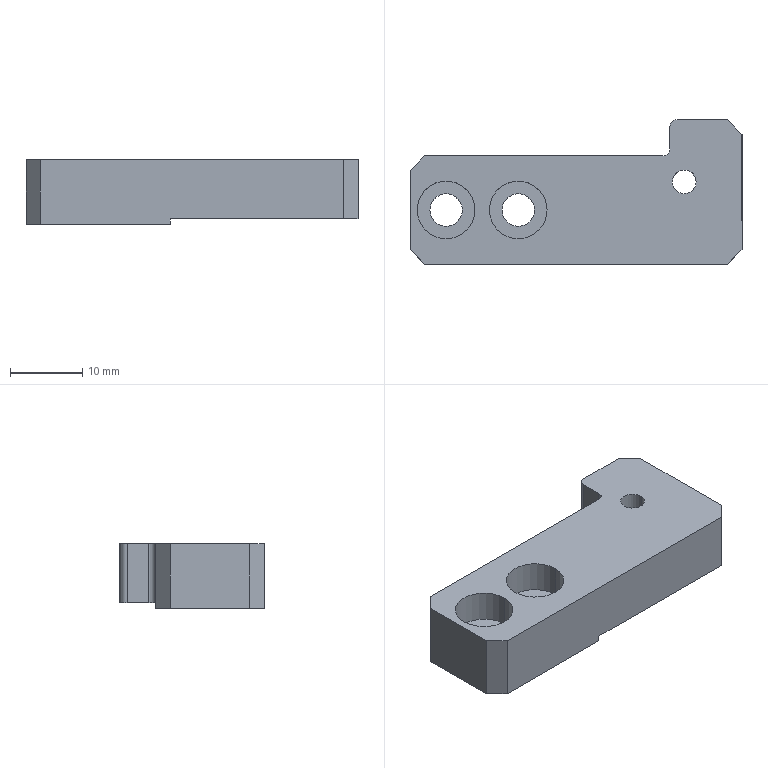Part | STEP file | 11-FG-B03811 | 1 solid | 28 faces | box 46 x 20 x 9 mm | volume 5580 mm3 | plane 16 | cylinder 12 | commonest cylinder face diameters 4.5 x4 8 x4 2 x2 3.3 x2
STEP:
#1=CARTESIAN_POINT('',(1.,7.5,4.6));
#2=VERTEX_POINT('',#1);
#3=CARTESIAN_POINT('',(9.,7.5,4.6));
#4=VERTEX_POINT('',#3);
#5=CARTESIAN_POINT('',(5.,7.5,4.6));
#6=DIRECTION('',(0.,0.,1.));
#7=DIRECTION('',(1.,0.,0.));
#8=AXIS2_PLACEMENT_3D('',#5,#6,#7);
#9=CIRCLE('',#8,4.);
#10=EDGE_CURVE('',#2,#4,#9,.T.);
#11=ORIENTED_EDGE('',*,*,#10,.F.);
#12=CARTESIAN_POINT('',(1.,7.5,9.));
#13=VERTEX_POINT('',#12);
#14=CARTESIAN_POINT('',(1.,7.5,9.));
#15=DIRECTION('',(0.,0.,1.));
#16=VECTOR('',#15,1000.);
#17=LINE('',#14,#16);
#18=EDGE_CURVE('',#2,#13,#17,.T.);
#19=ORIENTED_EDGE('',*,*,#18,.T.);
#20=CARTESIAN_POINT('',(9.,7.5,9.));
#21=VERTEX_POINT('',#20);
#22=CARTESIAN_POINT('',(5.,7.5,9.));
#23=DIRECTION('',(0.,0.,1.));
#24=DIRECTION('',(1.,0.,0.));
#25=AXIS2_PLACEMENT_3D('',#22,#23,#24);
#26=CIRCLE('',#25,4.);
#27=EDGE_CURVE('',#13,#21,#26,.T.);
#28=ORIENTED_EDGE('',*,*,#27,.T.);
#29=CARTESIAN_POINT('',(9.,7.5,9.));
#30=DIRECTION('',(0.,0.,1.));
#31=VECTOR('',#30,1000.);
#32=LINE('',#29,#31);
#33=EDGE_CURVE('',#4,#21,#32,.T.);
#34=ORIENTED_EDGE('',*,*,#33,.F.);
#35=EDGE_LOOP('',(#11,#19,#28,#34));
#36=FACE_OUTER_BOUND('',#35,.T.);
#37=CARTESIAN_POINT('',(5.,7.5,9.));
#38=DIRECTION('',(0.,0.,1.));
#39=DIRECTION('',(1.,0.,0.));
#40=AXIS2_PLACEMENT_3D('',#37,#38,#39);
#41=CYLINDRICAL_SURFACE('',#40,4.);
#42=ADVANCED_FACE('',(#36),#41,.F.);
#43=CARTESIAN_POINT('',(7.25,7.5,0.));
#44=VERTEX_POINT('',#43);
#45=CARTESIAN_POINT('',(2.75,7.5,0.));
#46=VERTEX_POINT('',#45);
#47=CARTESIAN_POINT('',(5.,7.5,0.));
#48=DIRECTION('',(0.,0.,-1.));
#49=DIRECTION('',(-1.,0.,0.));
#50=AXIS2_PLACEMENT_3D('',#47,#48,#49);
#51=CIRCLE('',#50,2.25);
#52=EDGE_CURVE('',#44,#46,#51,.T.);
#53=ORIENTED_EDGE('',*,*,#52,.T.);
#54=CARTESIAN_POINT('',(2.75,7.5,4.6));
#55=VERTEX_POINT('',#54);
#56=CARTESIAN_POINT('',(2.75,7.5,9.));
#57=DIRECTION('',(0.,0.,1.));
#58=VECTOR('',#57,1000.);
#59=LINE('',#56,#58);
#60=EDGE_CURVE('',#46,#55,#59,.T.);
#61=ORIENTED_EDGE('',*,*,#60,.T.);
#62=CARTESIAN_POINT('',(7.25,7.5,4.6));
#63=VERTEX_POINT('',#62);
#64=CARTESIAN_POINT('',(5.,7.5,4.6));
#65=DIRECTION('',(0.,0.,1.));
#66=DIRECTION('',(1.,0.,0.));
#67=AXIS2_PLACEMENT_3D('',#64,#65,#66);
#68=CIRCLE('',#67,2.25);
#69=EDGE_CURVE('',#55,#63,#68,.T.);
#70=ORIENTED_EDGE('',*,*,#69,.T.);
#71=CARTESIAN_POINT('',(7.25,7.5,9.));
#72=DIRECTION('',(0.,0.,1.));
#73=VECTOR('',#72,1000.);
#74=LINE('',#71,#73);
#75=EDGE_CURVE('',#44,#63,#74,.T.);
#76=ORIENTED_EDGE('',*,*,#75,.F.);
#77=EDGE_LOOP('',(#53,#61,#70,#76));
#78=FACE_OUTER_BOUND('',#77,.T.);
#79=CARTESIAN_POINT('',(5.,7.5,9.));
#80=DIRECTION('',(0.,0.,1.));
#81=DIRECTION('',(1.,0.,0.));
#82=AXIS2_PLACEMENT_3D('',#79,#80,#81);
#83=CYLINDRICAL_SURFACE('',#82,2.25);
#84=ADVANCED_FACE('',(#78),#83,.F.);
#85=CARTESIAN_POINT('',(11.,7.5,4.6));
#86=VERTEX_POINT('',#85);
#87=CARTESIAN_POINT('',(19.,7.5,4.6));
#88=VERTEX_POINT('',#87);
#89=CARTESIAN_POINT('',(15.,7.5,4.6));
#90=DIRECTION('',(0.,0.,1.));
#91=DIRECTION('',(1.,0.,0.));
#92=AXIS2_PLACEMENT_3D('',#89,#90,#91);
#93=CIRCLE('',#92,4.);
#94=EDGE_CURVE('',#86,#88,#93,.T.);
#95=ORIENTED_EDGE('',*,*,#94,.F.);
#96=CARTESIAN_POINT('',(11.,7.5,9.));
#97=VERTEX_POINT('',#96);
#98=CARTESIAN_POINT('',(11.,7.5,9.));
#99=DIRECTION('',(0.,0.,1.));
#100=VECTOR('',#99,1000.);
#101=LINE('',#98,#100);
#102=EDGE_CURVE('',#86,#97,#101,.T.);
#103=ORIENTED_EDGE('',*,*,#102,.T.);
#104=CARTESIAN_POINT('',(19.,7.5,9.));
#105=VERTEX_POINT('',#104);
#106=CARTESIAN_POINT('',(15.,7.5,9.));
#107=DIRECTION('',(0.,0.,1.));
#108=DIRECTION('',(1.,0.,0.));
#109=AXIS2_PLACEMENT_3D('',#106,#107,#108);
#110=CIRCLE('',#109,4.);
#111=EDGE_CURVE('',#97,#105,#110,.T.);
#112=ORIENTED_EDGE('',*,*,#111,.T.);
#113=CARTESIAN_POINT('',(19.,7.5,9.));
#114=DIRECTION('',(0.,0.,1.));
#115=VECTOR('',#114,1000.);
#116=LINE('',#113,#115);
#117=EDGE_CURVE('',#88,#105,#116,.T.);
#118=ORIENTED_EDGE('',*,*,#117,.F.);
#119=EDGE_LOOP('',(#95,#103,#112,#118));
#120=FACE_OUTER_BOUND('',#119,.T.);
#121=CARTESIAN_POINT('',(15.,7.5,9.));
#122=DIRECTION('',(0.,0.,1.));
#123=DIRECTION('',(1.,0.,0.));
#124=AXIS2_PLACEMENT_3D('',#121,#122,#123);
#125=CYLINDRICAL_SURFACE('',#124,4.);
#126=ADVANCED_FACE('',(#120),#125,.F.);
#127=CARTESIAN_POINT('',(17.25,7.5,0.));
#128=VERTEX_POINT('',#127);
#129=CARTESIAN_POINT('',(12.75,7.5,0.));
#130=VERTEX_POINT('',#129);
#131=CARTESIAN_POINT('',(15.,7.5,0.));
#132=DIRECTION('',(0.,0.,-1.));
#133=DIRECTION('',(-1.,0.,0.));
#134=AXIS2_PLACEMENT_3D('',#131,#132,#133);
#135=CIRCLE('',#134,2.25);
#136=EDGE_CURVE('',#128,#130,#135,.T.);
#137=ORIENTED_EDGE('',*,*,#136,.T.);
#138=CARTESIAN_POINT('',(12.75,7.5,4.6));
#139=VERTEX_POINT('',#138);
#140=CARTESIAN_POINT('',(12.75,7.5,9.));
#141=DIRECTION('',(0.,0.,1.));
#142=VECTOR('',#141,1000.);
#143=LINE('',#140,#142);
#144=EDGE_CURVE('',#130,#139,#143,.T.);
#145=ORIENTED_EDGE('',*,*,#144,.T.);
#146=CARTESIAN_POINT('',(17.25,7.5,4.6));
#147=VERTEX_POINT('',#146);
#148=CARTESIAN_POINT('',(15.,7.5,4.6));
#149=DIRECTION('',(0.,0.,1.));
#150=DIRECTION('',(1.,0.,0.));
#151=AXIS2_PLACEMENT_3D('',#148,#149,#150);
#152=CIRCLE('',#151,2.25);
#153=EDGE_CURVE('',#139,#147,#152,.T.);
#154=ORIENTED_EDGE('',*,*,#153,.T.);
#155=CARTESIAN_POINT('',(17.25,7.5,9.));
#156=DIRECTION('',(0.,0.,1.));
#157=VECTOR('',#156,1000.);
#158=LINE('',#155,#157);
#159=EDGE_CURVE('',#128,#147,#158,.T.);
#160=ORIENTED_EDGE('',*,*,#159,.F.);
#161=EDGE_LOOP('',(#137,#145,#154,#160));
#162=FACE_OUTER_BOUND('',#161,.T.);
#163=CARTESIAN_POINT('',(15.,7.5,9.));
#164=DIRECTION('',(0.,0.,1.));
#165=DIRECTION('',(1.,0.,0.));
#166=AXIS2_PLACEMENT_3D('',#163,#164,#165);
#167=CYLINDRICAL_SURFACE('',#166,2.25);
#168=ADVANCED_FACE('',(#162),#167,.F.);
#169=CARTESIAN_POINT('',(39.65,11.4,9.));
#170=VERTEX_POINT('',#169);
#171=CARTESIAN_POINT('',(36.35,11.4,9.));
#172=VERTEX_POINT('',#171);
#173=CARTESIAN_POINT('',(38.,11.4,9.));
#174=DIRECTION('',(0.,0.,-1.));
#175=DIRECTION('',(-1.,0.,0.));
#176=AXIS2_PLACEMENT_3D('',#173,#174,#175);
#177=CIRCLE('',#176,1.65);
#178=EDGE_CURVE('',#170,#172,#177,.T.);
#179=ORIENTED_EDGE('',*,*,#178,.F.);
#180=CARTESIAN_POINT('',(39.65,11.4,0.8));
#181=VERTEX_POINT('',#180);
#182=CARTESIAN_POINT('',(39.65,11.4,0.));
#183=DIRECTION('',(0.,0.,-1.));
#184=VECTOR('',#183,1000.);
#185=LINE('',#182,#184);
#186=EDGE_CURVE('',#170,#181,#185,.T.);
#187=ORIENTED_EDGE('',*,*,#186,.T.);
#188=CARTESIAN_POINT('',(36.35,11.4,0.8));
#189=VERTEX_POINT('',#188);
#190=CARTESIAN_POINT('',(38.,11.4,0.8));
#191=DIRECTION('',(0.,0.,-1.));
#192=DIRECTION('',(1.,0.,0.));
#193=AXIS2_PLACEMENT_3D('',#190,#191,#192);
#194=CIRCLE('',#193,1.65);
#195=EDGE_CURVE('',#181,#189,#194,.T.);
#196=ORIENTED_EDGE('',*,*,#195,.T.);
#197=CARTESIAN_POINT('',(36.35,11.4,0.));
#198=DIRECTION('',(0.,0.,-1.));
#199=VECTOR('',#198,1000.);
#200=LINE('',#197,#199);
#201=EDGE_CURVE('',#172,#189,#200,.T.);
#202=ORIENTED_EDGE('',*,*,#201,.F.);
#203=EDGE_LOOP('',(#179,#187,#196,#202));
#204=FACE_OUTER_BOUND('',#203,.T.);
#205=CARTESIAN_POINT('',(38.,11.4,0.));
#206=DIRECTION('',(0.,0.,-1.));
#207=DIRECTION('',(-1.,0.,0.));
#208=AXIS2_PLACEMENT_3D('',#205,#206,#207);
#209=CYLINDRICAL_SURFACE('',#208,1.65);
#210=ADVANCED_FACE('',(#204),#209,.F.);
#211=CARTESIAN_POINT('',(0.,13.,9.));
#212=VERTEX_POINT('',#211);
#213=CARTESIAN_POINT('',(0.,2.,9.));
#214=VERTEX_POINT('',#213);
#215=CARTESIAN_POINT('',(0.,0.,9.));
#216=DIRECTION('',(0.,-1.,0.));
#217=VECTOR('',#216,1000.);
#218=LINE('',#215,#217);
#219=EDGE_CURVE('',#212,#214,#218,.T.);
#220=ORIENTED_EDGE('',*,*,#219,.F.);
#221=CARTESIAN_POINT('',(0.,13.,0.));
#222=VERTEX_POINT('',#221);
#223=CARTESIAN_POINT('',(0.,13.,9.));
#224=DIRECTION('',(0.,0.,-1.));
#225=VECTOR('',#224,1000.);
#226=LINE('',#223,#225);
#227=EDGE_CURVE('',#212,#222,#226,.T.);
#228=ORIENTED_EDGE('',*,*,#227,.T.);
#229=CARTESIAN_POINT('',(0.,2.,0.));
#230=VERTEX_POINT('',#229);
#231=CARTESIAN_POINT('',(0.,0.,0.));
#232=DIRECTION('',(0.,-1.,0.));
#233=VECTOR('',#232,1000.);
#234=LINE('',#231,#233);
#235=EDGE_CURVE('',#222,#230,#234,.T.);
#236=ORIENTED_EDGE('',*,*,#235,.T.);
#237=CARTESIAN_POINT('',(0.,2.,9.));
#238=DIRECTION('',(0.,0.,1.));
#239=VECTOR('',#238,1000.);
#240=LINE('',#237,#239);
#241=EDGE_CURVE('',#230,#214,#240,.T.);
#242=ORIENTED_EDGE('',*,*,#241,.T.);
#243=EDGE_LOOP('',(#220,#228,#236,#242));
#244=FACE_OUTER_BOUND('',#243,.T.);
#245=CARTESIAN_POINT('',(0.,0.,9.));
#246=DIRECTION('',(1.,0.,0.));
#247=DIRECTION('',(0.,1.,0.));
#248=AXIS2_PLACEMENT_3D('',#245,#246,#247);
#249=PLANE('',#248);
#250=ADVANCED_FACE('',(#244),#249,.F.);
#251=CARTESIAN_POINT('',(2.,0.,0.));
#252=VERTEX_POINT('',#251);
#253=CARTESIAN_POINT('',(20.,0.,0.));
#254=VERTEX_POINT('',#253);
#255=CARTESIAN_POINT('',(0.,0.,0.));
#256=DIRECTION('',(1.,0.,0.));
#257=VECTOR('',#256,1000.);
#258=LINE('',#255,#257);
#259=EDGE_CURVE('',#252,#254,#258,.T.);
#260=ORIENTED_EDGE('',*,*,#259,.T.);
#261=CARTESIAN_POINT('',(20.,0.,0.8));
#262=VERTEX_POINT('',#261);
#263=CARTESIAN_POINT('',(20.,0.,0.));
#264=DIRECTION('',(0.,0.,-1.));
#265=VECTOR('',#264,1000.);
#266=LINE('',#263,#265);
#267=EDGE_CURVE('',#262,#254,#266,.T.);
#268=ORIENTED_EDGE('',*,*,#267,.F.);
#269=CARTESIAN_POINT('',(44.,0.,0.8));
#270=VERTEX_POINT('',#269);
#271=CARTESIAN_POINT('',(46.,0.,0.8));
#272=DIRECTION('',(-1.,0.,0.));
#273=VECTOR('',#272,1000.);
#274=LINE('',#271,#273);
#275=EDGE_CURVE('',#270,#262,#274,.T.);
#276=ORIENTED_EDGE('',*,*,#275,.F.);
#277=CARTESIAN_POINT('',(44.,0.,9.));
#278=VERTEX_POINT('',#277);
#279=CARTESIAN_POINT('',(44.,0.,9.));
#280=DIRECTION('',(0.,0.,1.));
#281=VECTOR('',#280,1000.);
#282=LINE('',#279,#281);
#283=EDGE_CURVE('',#270,#278,#282,.T.);
#284=ORIENTED_EDGE('',*,*,#283,.T.);
#285=CARTESIAN_POINT('',(2.,0.,9.));
#286=VERTEX_POINT('',#285);
#287=CARTESIAN_POINT('',(0.,0.,9.));
#288=DIRECTION('',(1.,0.,0.));
#289=VECTOR('',#288,1000.);
#290=LINE('',#287,#289);
#291=EDGE_CURVE('',#286,#278,#290,.T.);
#292=ORIENTED_EDGE('',*,*,#291,.F.);
#293=CARTESIAN_POINT('',(2.,0.,9.));
#294=DIRECTION('',(0.,0.,-1.));
#295=VECTOR('',#294,1000.);
#296=LINE('',#293,#295);
#297=EDGE_CURVE('',#286,#252,#296,.T.);
#298=ORIENTED_EDGE('',*,*,#297,.T.);
#299=EDGE_LOOP('',(#260,#268,#276,#284,#292,#298));
#300=FACE_OUTER_BOUND('',#299,.T.);
#301=CARTESIAN_POINT('',(0.,0.,9.));
#302=DIRECTION('',(0.,1.,0.));
#303=DIRECTION('',(0.,0.,1.));
#304=AXIS2_PLACEMENT_3D('',#301,#302,#303);
#305=PLANE('',#304);
#306=ADVANCED_FACE('',(#300),#305,.F.);
#307=CARTESIAN_POINT('',(46.,2.,9.));
#308=VERTEX_POINT('',#307);
#309=CARTESIAN_POINT('',(46.,2.,0.8));
#310=VERTEX_POINT('',#309);
#311=CARTESIAN_POINT('',(46.,2.,9.));
#312=DIRECTION('',(0.,0.,-1.));
#313=VECTOR('',#312,1000.);
#314=LINE('',#311,#313);
#315=EDGE_CURVE('',#308,#310,#314,.T.);
#316=ORIENTED_EDGE('',*,*,#315,.T.);
#317=CARTESIAN_POINT('',(46.,18.,0.8));
#318=VERTEX_POINT('',#317);
#319=CARTESIAN_POINT('',(46.,29.,0.8));
#320=DIRECTION('',(0.,-1.,0.));
#321=VECTOR('',#320,1000.);
#322=LINE('',#319,#321);
#323=EDGE_CURVE('',#318,#310,#322,.T.);
#324=ORIENTED_EDGE('',*,*,#323,.F.);
#325=CARTESIAN_POINT('',(46.,18.,9.));
#326=VERTEX_POINT('',#325);
#327=CARTESIAN_POINT('',(46.,18.,9.));
#328=DIRECTION('',(0.,0.,1.));
#329=VECTOR('',#328,1000.);
#330=LINE('',#327,#329);
#331=EDGE_CURVE('',#318,#326,#330,.T.);
#332=ORIENTED_EDGE('',*,*,#331,.T.);
#333=CARTESIAN_POINT('',(46.,0.,9.));
#334=DIRECTION('',(0.,1.,0.));
#335=VECTOR('',#334,1000.);
#336=LINE('',#333,#335);
#337=EDGE_CURVE('',#308,#326,#336,.T.);
#338=ORIENTED_EDGE('',*,*,#337,.F.);
#339=EDGE_LOOP('',(#316,#324,#332,#338));
#340=FACE_OUTER_BOUND('',#339,.T.);
#341=CARTESIAN_POINT('',(46.,0.,9.));
#342=DIRECTION('',(-1.,0.,0.));
#343=DIRECTION('',(0.,-1.,0.));
#344=AXIS2_PLACEMENT_3D('',#341,#342,#343);
#345=PLANE('',#344);
#346=ADVANCED_FACE('',(#340),#345,.F.);
#347=CARTESIAN_POINT('',(44.,20.,0.8));
#348=VERTEX_POINT('',#347);
#349=CARTESIAN_POINT('',(37.,20.,0.8));
#350=VERTEX_POINT('',#349);
#351=CARTESIAN_POINT('',(0.,20.,0.8));
#352=DIRECTION('',(-1.,0.,0.));
#353=VECTOR('',#352,1000.);
#354=LINE('',#351,#353);
#355=EDGE_CURVE('',#348,#350,#354,.T.);
#356=ORIENTED_EDGE('',*,*,#355,.T.);
#357=CARTESIAN_POINT('',(37.,20.,9.));
#358=VERTEX_POINT('',#357);
#359=CARTESIAN_POINT('',(37.,20.,9.));
#360=DIRECTION('',(0.,0.,1.));
#361=VECTOR('',#360,1000.);
#362=LINE('',#359,#361);
#363=EDGE_CURVE('',#350,#358,#362,.T.);
#364=ORIENTED_EDGE('',*,*,#363,.T.);
#365=CARTESIAN_POINT('',(44.,20.,9.));
#366=VERTEX_POINT('',#365);
#367=CARTESIAN_POINT('',(0.,20.,9.));
#368=DIRECTION('',(-1.,0.,0.));
#369=VECTOR('',#368,1000.);
#370=LINE('',#367,#369);
#371=EDGE_CURVE('',#366,#358,#370,.T.);
#372=ORIENTED_EDGE('',*,*,#371,.F.);
#373=CARTESIAN_POINT('',(44.,20.,9.));
#374=DIRECTION('',(0.,0.,-1.));
#375=VECTOR('',#374,1000.);
#376=LINE('',#373,#375);
#377=EDGE_CURVE('',#366,#348,#376,.T.);
#378=ORIENTED_EDGE('',*,*,#377,.T.);
#379=EDGE_LOOP('',(#356,#364,#372,#378));
#380=FACE_OUTER_BOUND('',#379,.T.);
#381=CARTESIAN_POINT('',(0.,20.,9.));
#382=DIRECTION('',(0.,-1.,0.));
#383=DIRECTION('',(0.,0.,-1.));
#384=AXIS2_PLACEMENT_3D('',#381,#382,#383);
#385=PLANE('',#384);
#386=ADVANCED_FACE('',(#380),#385,.F.);
#387=CARTESIAN_POINT('',(5.,7.5,9.));
#388=DIRECTION('',(0.,0.,1.));
#389=DIRECTION('',(1.,0.,0.));
#390=AXIS2_PLACEMENT_3D('',#387,#388,#389);
#391=CIRCLE('',#390,4.);
#392=EDGE_CURVE('',#21,#13,#391,.T.);
#393=ORIENTED_EDGE('',*,*,#392,.F.);
#394=ORIENTED_EDGE('',*,*,#27,.F.);
#395=EDGE_LOOP('',(#393,#394));
#396=FACE_BOUND('',#395,.T.);
#397=CARTESIAN_POINT('',(15.,7.5,9.));
#398=DIRECTION('',(0.,0.,1.));
#399=DIRECTION('',(1.,0.,0.));
#400=AXIS2_PLACEMENT_3D('',#397,#398,#399);
#401=CIRCLE('',#400,4.);
#402=EDGE_CURVE('',#105,#97,#401,.T.);
#403=ORIENTED_EDGE('',*,*,#402,.F.);
#404=ORIENTED_EDGE('',*,*,#111,.F.);
#405=EDGE_LOOP('',(#403,#404));
#406=FACE_BOUND('',#405,.T.);
#407=CARTESIAN_POINT('',(38.,11.4,9.));
#408=DIRECTION('',(0.,0.,-1.));
#409=DIRECTION('',(-1.,0.,0.));
#410=AXIS2_PLACEMENT_3D('',#407,#408,#409);
#411=CIRCLE('',#410,1.65);
#412=EDGE_CURVE('',#172,#170,#411,.T.);
#413=ORIENTED_EDGE('',*,*,#412,.T.);
#414=ORIENTED_EDGE('',*,*,#178,.T.);
#415=EDGE_LOOP('',(#413,#414));
#416=FACE_BOUND('',#415,.T.);
#417=ORIENTED_EDGE('',*,*,#371,.T.);
#418=CARTESIAN_POINT('',(36.,19.,9.));
#419=VERTEX_POINT('',#418);
#420=CARTESIAN_POINT('',(37.,19.,9.));
#421=DIRECTION('',(0.,0.,1.));
#422=DIRECTION('',(-1.,0.,0.));
#423=AXIS2_PLACEMENT_3D('',#420,#421,#422);
#424=CIRCLE('',#423,1.);
#425=EDGE_CURVE('',#358,#419,#424,.T.);
#426=ORIENTED_EDGE('',*,*,#425,.T.);
#427=CARTESIAN_POINT('',(36.,16.,9.));
#428=VERTEX_POINT('',#427);
#429=CARTESIAN_POINT('',(36.,15.,9.));
#430=DIRECTION('',(0.,1.,0.));
#431=VECTOR('',#430,1000.);
#432=LINE('',#429,#431);
#433=EDGE_CURVE('',#428,#419,#432,.T.);
#434=ORIENTED_EDGE('',*,*,#433,.F.);
#435=CARTESIAN_POINT('',(35.,15.,9.));
#436=VERTEX_POINT('',#435);
#437=CARTESIAN_POINT('',(35.,16.,9.));
#438=DIRECTION('',(0.,0.,-1.));
#439=DIRECTION('',(-1.,0.,0.));
#440=AXIS2_PLACEMENT_3D('',#437,#438,#439);
#441=CIRCLE('',#440,1.);
#442=EDGE_CURVE('',#428,#436,#441,.T.);
#443=ORIENTED_EDGE('',*,*,#442,.T.);
#444=CARTESIAN_POINT('',(2.,15.,9.));
#445=VERTEX_POINT('',#444);
#446=CARTESIAN_POINT('',(0.,15.,9.));
#447=DIRECTION('',(1.,0.,0.));
#448=VECTOR('',#447,1000.);
#449=LINE('',#446,#448);
#450=EDGE_CURVE('',#445,#436,#449,.T.);
#451=ORIENTED_EDGE('',*,*,#450,.F.);
#452=CARTESIAN_POINT('',(2.,15.,9.));
#453=DIRECTION('',(-0.7071,-0.7071,0.));
#454=VECTOR('',#453,1000.);
#455=LINE('',#452,#454);
#456=EDGE_CURVE('',#445,#212,#455,.T.);
#457=ORIENTED_EDGE('',*,*,#456,.T.);
#458=ORIENTED_EDGE('',*,*,#219,.T.);
#459=CARTESIAN_POINT('',(2.,0.,9.));
#460=DIRECTION('',(0.7071,-0.7071,0.));
#461=VECTOR('',#460,1000.);
#462=LINE('',#459,#461);
#463=EDGE_CURVE('',#214,#286,#462,.T.);
#464=ORIENTED_EDGE('',*,*,#463,.T.);
#465=ORIENTED_EDGE('',*,*,#291,.T.);
#466=CARTESIAN_POINT('',(46.,2.,9.));
#467=DIRECTION('',(0.7071,0.7071,0.));
#468=VECTOR('',#467,1000.);
#469=LINE('',#466,#468);
#470=EDGE_CURVE('',#278,#308,#469,.T.);
#471=ORIENTED_EDGE('',*,*,#470,.T.);
#472=ORIENTED_EDGE('',*,*,#337,.T.);
#473=CARTESIAN_POINT('',(44.,20.,9.));
#474=DIRECTION('',(-0.7071,0.7071,0.));
#475=VECTOR('',#474,1000.);
#476=LINE('',#473,#475);
#477=EDGE_CURVE('',#326,#366,#476,.T.);
#478=ORIENTED_EDGE('',*,*,#477,.T.);
#479=EDGE_LOOP('',(#417,#426,#434,#443,#451,#457,#458,#464,#465,#471,#472,#478));
#480=FACE_OUTER_BOUND('',#479,.T.);
#481=CARTESIAN_POINT('',(0.,20.,9.));
#482=DIRECTION('',(0.,0.,-1.));
#483=DIRECTION('',(-1.,0.,0.));
#484=AXIS2_PLACEMENT_3D('',#481,#482,#483);
#485=PLANE('',#484);
#486=ADVANCED_FACE('',(#396,#406,#416,#480),#485,.F.);
#487=CARTESIAN_POINT('',(20.,15.,0.));
#488=VERTEX_POINT('',#487);
#489=CARTESIAN_POINT('',(20.,29.,0.));
#490=DIRECTION('',(0.,-1.,0.));
#491=VECTOR('',#490,1000.);
#492=LINE('',#489,#491);
#493=EDGE_CURVE('',#488,#254,#492,.T.);
#494=ORIENTED_EDGE('',*,*,#493,.T.);
#495=ORIENTED_EDGE('',*,*,#259,.F.);
#496=CARTESIAN_POINT('',(-9.,11.,0.));
#497=DIRECTION('',(-0.7071,0.7071,0.));
#498=VECTOR('',#497,1000.);
#499=LINE('',#496,#498);
#500=EDGE_CURVE('',#252,#230,#499,.T.);
#501=ORIENTED_EDGE('',*,*,#500,.T.);
#502=ORIENTED_EDGE('',*,*,#235,.F.);
#503=CARTESIAN_POINT('',(2.,15.,0.));
#504=VERTEX_POINT('',#503);
#505=CARTESIAN_POINT('',(3.5,16.5,0.));
#506=DIRECTION('',(0.7071,0.7071,0.));
#507=VECTOR('',#506,1000.);
#508=LINE('',#505,#507);
#509=EDGE_CURVE('',#222,#504,#508,.T.);
#510=ORIENTED_EDGE('',*,*,#509,.T.);
#511=CARTESIAN_POINT('',(0.,15.,0.));
#512=DIRECTION('',(-1.,0.,0.));
#513=VECTOR('',#512,1000.);
#514=LINE('',#511,#513);
#515=EDGE_CURVE('',#488,#504,#514,.T.);
#516=ORIENTED_EDGE('',*,*,#515,.F.);
#517=EDGE_LOOP('',(#494,#495,#501,#502,#510,#516));
#518=FACE_OUTER_BOUND('',#517,.T.);
#519=ORIENTED_EDGE('',*,*,#52,.F.);
#520=CARTESIAN_POINT('',(5.,7.5,0.));
#521=DIRECTION('',(0.,0.,-1.));
#522=DIRECTION('',(-1.,0.,0.));
#523=AXIS2_PLACEMENT_3D('',#520,#521,#522);
#524=CIRCLE('',#523,2.25);
#525=EDGE_CURVE('',#46,#44,#524,.T.);
#526=ORIENTED_EDGE('',*,*,#525,.F.);
#527=EDGE_LOOP('',(#519,#526));
#528=FACE_BOUND('',#527,.T.);
#529=ORIENTED_EDGE('',*,*,#136,.F.);
#530=CARTESIAN_POINT('',(15.,7.5,0.));
#531=DIRECTION('',(0.,0.,-1.));
#532=DIRECTION('',(-1.,0.,0.));
#533=AXIS2_PLACEMENT_3D('',#530,#531,#532);
#534=CIRCLE('',#533,2.25);
#535=EDGE_CURVE('',#130,#128,#534,.T.);
#536=ORIENTED_EDGE('',*,*,#535,.F.);
#537=EDGE_LOOP('',(#529,#536));
#538=FACE_BOUND('',#537,.T.);
#539=CARTESIAN_POINT('',(0.,20.,0.));
#540=DIRECTION('',(0.,0.,-1.));
#541=DIRECTION('',(-1.,0.,0.));
#542=AXIS2_PLACEMENT_3D('',#539,#540,#541);
#543=PLANE('',#542);
#544=ADVANCED_FACE('',(#518,#528,#538),#543,.T.);
#545=ORIENTED_EDGE('',*,*,#450,.T.);
#546=CARTESIAN_POINT('',(35.,15.,0.8));
#547=VERTEX_POINT('',#546);
#548=CARTESIAN_POINT('',(35.,15.,0.8));
#549=DIRECTION('',(0.,0.,-1.));
#550=VECTOR('',#549,1000.);
#551=LINE('',#548,#550);
#552=EDGE_CURVE('',#436,#547,#551,.T.);
#553=ORIENTED_EDGE('',*,*,#552,.T.);
#554=CARTESIAN_POINT('',(20.,15.,0.8));
#555=VERTEX_POINT('',#554);
#556=CARTESIAN_POINT('',(0.,15.,0.8));
#557=DIRECTION('',(-1.,0.,0.));
#558=VECTOR('',#557,1000.);
#559=LINE('',#556,#558);
#560=EDGE_CURVE('',#547,#555,#559,.T.);
#561=ORIENTED_EDGE('',*,*,#560,.T.);
#562=CARTESIAN_POINT('',(20.,15.,-7.));
#563=DIRECTION('',(0.,0.,-1.));
#564=VECTOR('',#563,1000.);
#565=LINE('',#562,#564);
#566=EDGE_CURVE('',#555,#488,#565,.T.);
#567=ORIENTED_EDGE('',*,*,#566,.T.);
#568=ORIENTED_EDGE('',*,*,#515,.T.);
#569=CARTESIAN_POINT('',(2.,15.,-7.));
#570=DIRECTION('',(0.,0.,1.));
#571=VECTOR('',#570,1000.);
#572=LINE('',#569,#571);
#573=EDGE_CURVE('',#504,#445,#572,.T.);
#574=ORIENTED_EDGE('',*,*,#573,.T.);
#575=EDGE_LOOP('',(#545,#553,#561,#567,#568,#574));
#576=FACE_OUTER_BOUND('',#575,.T.);
#577=CARTESIAN_POINT('',(0.,15.,-7.));
#578=DIRECTION('',(0.,-1.,0.));
#579=DIRECTION('',(1.,0.,0.));
#580=AXIS2_PLACEMENT_3D('',#577,#578,#579);
#581=PLANE('',#580);
#582=ADVANCED_FACE('',(#576),#581,.F.);
#583=ORIENTED_EDGE('',*,*,#186,.F.);
#584=ORIENTED_EDGE('',*,*,#412,.F.);
#585=ORIENTED_EDGE('',*,*,#201,.T.);
#586=CARTESIAN_POINT('',(38.,11.4,0.8));
#587=DIRECTION('',(0.,0.,-1.));
#588=DIRECTION('',(1.,0.,0.));
#589=AXIS2_PLACEMENT_3D('',#586,#587,#588);
#590=CIRCLE('',#589,1.65);
#591=EDGE_CURVE('',#189,#181,#590,.T.);
#592=ORIENTED_EDGE('',*,*,#591,.T.);
#593=EDGE_LOOP('',(#583,#584,#585,#592));
#594=FACE_OUTER_BOUND('',#593,.T.);
#595=CARTESIAN_POINT('',(38.,11.4,0.));
#596=DIRECTION('',(0.,0.,-1.));
#597=DIRECTION('',(-1.,0.,0.));
#598=AXIS2_PLACEMENT_3D('',#595,#596,#597);
#599=CYLINDRICAL_SURFACE('',#598,1.65);
#600=ADVANCED_FACE('',(#594),#599,.F.);
#601=ORIENTED_EDGE('',*,*,#144,.F.);
#602=ORIENTED_EDGE('',*,*,#535,.T.);
#603=ORIENTED_EDGE('',*,*,#159,.T.);
#604=CARTESIAN_POINT('',(15.,7.5,4.6));
#605=DIRECTION('',(0.,0.,1.));
#606=DIRECTION('',(1.,0.,0.));
#607=AXIS2_PLACEMENT_3D('',#604,#605,#606);
#608=CIRCLE('',#607,2.25);
#609=EDGE_CURVE('',#147,#139,#608,.T.);
#610=ORIENTED_EDGE('',*,*,#609,.T.);
#611=EDGE_LOOP('',(#601,#602,#603,#610));
#612=FACE_OUTER_BOUND('',#611,.T.);
#613=CARTESIAN_POINT('',(15.,7.5,9.));
#614=DIRECTION('',(0.,0.,1.));
#615=DIRECTION('',(1.,0.,0.));
#616=AXIS2_PLACEMENT_3D('',#613,#614,#615);
#617=CYLINDRICAL_SURFACE('',#616,2.25);
#618=ADVANCED_FACE('',(#612),#617,.F.);
#619=ORIENTED_EDGE('',*,*,#609,.F.);
#620=ORIENTED_EDGE('',*,*,#153,.F.);
#621=EDGE_LOOP('',(#619,#620));
#622=FACE_BOUND('',#621,.T.);
#623=CARTESIAN_POINT('',(15.,7.5,4.6));
#624=DIRECTION('',(0.,0.,1.));
#625=DIRECTION('',(1.,0.,0.));
#626=AXIS2_PLACEMENT_3D('',#623,#624,#625);
#627=CIRCLE('',#626,4.);
#628=EDGE_CURVE('',#88,#86,#627,.T.);
#629=ORIENTED_EDGE('',*,*,#628,.T.);
#630=ORIENTED_EDGE('',*,*,#94,.T.);
#631=EDGE_LOOP('',(#629,#630));
#632=FACE_OUTER_BOUND('',#631,.T.);
#633=CARTESIAN_POINT('',(17.25,7.5,4.6));
#634=DIRECTION('',(0.,0.,-1.));
#635=DIRECTION('',(-1.,0.,0.));
#636=AXIS2_PLACEMENT_3D('',#633,#634,#635);
#637=PLANE('',#636);
#638=ADVANCED_FACE('',(#622,#632),#637,.F.);
#639=ORIENTED_EDGE('',*,*,#102,.F.);
#640=ORIENTED_EDGE('',*,*,#628,.F.);
#641=ORIENTED_EDGE('',*,*,#117,.T.);
#642=ORIENTED_EDGE('',*,*,#402,.T.);
#643=EDGE_LOOP('',(#639,#640,#641,#642));
#644=FACE_OUTER_BOUND('',#643,.T.);
#645=CARTESIAN_POINT('',(15.,7.5,9.));
#646=DIRECTION('',(0.,0.,1.));
#647=DIRECTION('',(1.,0.,0.));
#648=AXIS2_PLACEMENT_3D('',#645,#646,#647);
#649=CYLINDRICAL_SURFACE('',#648,4.);
#650=ADVANCED_FACE('',(#644),#649,.F.);
#651=ORIENTED_EDGE('',*,*,#60,.F.);
#652=ORIENTED_EDGE('',*,*,#525,.T.);
#653=ORIENTED_EDGE('',*,*,#75,.T.);
#654=CARTESIAN_POINT('',(5.,7.5,4.6));
#655=DIRECTION('',(0.,0.,1.));
#656=DIRECTION('',(1.,0.,0.));
#657=AXIS2_PLACEMENT_3D('',#654,#655,#656);
#658=CIRCLE('',#657,2.25);
#659=EDGE_CURVE('',#63,#55,#658,.T.);
#660=ORIENTED_EDGE('',*,*,#659,.T.);
#661=EDGE_LOOP('',(#651,#652,#653,#660));
#662=FACE_OUTER_BOUND('',#661,.T.);
#663=CARTESIAN_POINT('',(5.,7.5,9.));
#664=DIRECTION('',(0.,0.,1.));
#665=DIRECTION('',(1.,0.,0.));
#666=AXIS2_PLACEMENT_3D('',#663,#664,#665);
#667=CYLINDRICAL_SURFACE('',#666,2.25);
#668=ADVANCED_FACE('',(#662),#667,.F.);
#669=ORIENTED_EDGE('',*,*,#659,.F.);
#670=ORIENTED_EDGE('',*,*,#69,.F.);
#671=EDGE_LOOP('',(#669,#670));
#672=FACE_BOUND('',#671,.T.);
#673=CARTESIAN_POINT('',(5.,7.5,4.6));
#674=DIRECTION('',(0.,0.,1.));
#675=DIRECTION('',(1.,0.,0.));
#676=AXIS2_PLACEMENT_3D('',#673,#674,#675);
#677=CIRCLE('',#676,4.);
#678=EDGE_CURVE('',#4,#2,#677,.T.);
#679=ORIENTED_EDGE('',*,*,#678,.T.);
#680=ORIENTED_EDGE('',*,*,#10,.T.);
#681=EDGE_LOOP('',(#679,#680));
#682=FACE_OUTER_BOUND('',#681,.T.);
#683=CARTESIAN_POINT('',(7.25,7.5,4.6));
#684=DIRECTION('',(0.,0.,-1.));
#685=DIRECTION('',(-1.,0.,0.));
#686=AXIS2_PLACEMENT_3D('',#683,#684,#685);
#687=PLANE('',#686);
#688=ADVANCED_FACE('',(#672,#682),#687,.F.);
#689=ORIENTED_EDGE('',*,*,#18,.F.);
#690=ORIENTED_EDGE('',*,*,#678,.F.);
#691=ORIENTED_EDGE('',*,*,#33,.T.);
#692=ORIENTED_EDGE('',*,*,#392,.T.);
#693=EDGE_LOOP('',(#689,#690,#691,#692));
#694=FACE_OUTER_BOUND('',#693,.T.);
#695=CARTESIAN_POINT('',(5.,7.5,9.));
#696=DIRECTION('',(0.,0.,1.));
#697=DIRECTION('',(1.,0.,0.));
#698=AXIS2_PLACEMENT_3D('',#695,#696,#697);
#699=CYLINDRICAL_SURFACE('',#698,4.);
#700=ADVANCED_FACE('',(#694),#699,.F.);
#701=ORIENTED_EDGE('',*,*,#509,.F.);
#702=ORIENTED_EDGE('',*,*,#227,.F.);
#703=ORIENTED_EDGE('',*,*,#456,.F.);
#704=ORIENTED_EDGE('',*,*,#573,.F.);
#705=EDGE_LOOP('',(#701,#702,#703,#704));
#706=FACE_OUTER_BOUND('',#705,.T.);
#707=CARTESIAN_POINT('',(2.,15.,-7.));
#708=DIRECTION('',(0.7071,-0.7071,0.));
#709=DIRECTION('',(0.,0.,1.));
#710=AXIS2_PLACEMENT_3D('',#707,#708,#709);
#711=PLANE('',#710);
#712=ADVANCED_FACE('',(#706),#711,.F.);
#713=ORIENTED_EDGE('',*,*,#463,.F.);
#714=ORIENTED_EDGE('',*,*,#241,.F.);
#715=ORIENTED_EDGE('',*,*,#500,.F.);
#716=ORIENTED_EDGE('',*,*,#297,.F.);
#717=EDGE_LOOP('',(#713,#714,#715,#716));
#718=FACE_OUTER_BOUND('',#717,.T.);
#719=CARTESIAN_POINT('',(2.,0.,9.));
#720=DIRECTION('',(0.7071,0.7071,0.));
#721=DIRECTION('',(0.,0.,-1.));
#722=AXIS2_PLACEMENT_3D('',#719,#720,#721);
#723=PLANE('',#722);
#724=ADVANCED_FACE('',(#718),#723,.F.);
#725=CARTESIAN_POINT('',(46.,2.,0.8));
#726=DIRECTION('',(-0.7071,-0.7071,0.));
#727=VECTOR('',#726,1000.);
#728=LINE('',#725,#727);
#729=EDGE_CURVE('',#310,#270,#728,.T.);
#730=ORIENTED_EDGE('',*,*,#729,.F.);
#731=ORIENTED_EDGE('',*,*,#315,.F.);
#732=ORIENTED_EDGE('',*,*,#470,.F.);
#733=ORIENTED_EDGE('',*,*,#283,.F.);
#734=EDGE_LOOP('',(#730,#731,#732,#733));
#735=FACE_OUTER_BOUND('',#734,.T.);
#736=CARTESIAN_POINT('',(46.,2.,9.));
#737=DIRECTION('',(-0.7071,0.7071,0.));
#738=DIRECTION('',(0.,0.,-1.));
#739=AXIS2_PLACEMENT_3D('',#736,#737,#738);
#740=PLANE('',#739);
#741=ADVANCED_FACE('',(#735),#740,.F.);
#742=CARTESIAN_POINT('',(44.,20.,0.8));
#743=DIRECTION('',(0.7071,-0.7071,0.));
#744=VECTOR('',#743,1000.);
#745=LINE('',#742,#744);
#746=EDGE_CURVE('',#348,#318,#745,.T.);
#747=ORIENTED_EDGE('',*,*,#746,.F.);
#748=ORIENTED_EDGE('',*,*,#377,.F.);
#749=ORIENTED_EDGE('',*,*,#477,.F.);
#750=ORIENTED_EDGE('',*,*,#331,.F.);
#751=EDGE_LOOP('',(#747,#748,#749,#750));
#752=FACE_OUTER_BOUND('',#751,.T.);
#753=CARTESIAN_POINT('',(44.,20.,9.));
#754=DIRECTION('',(-0.7071,-0.7071,0.));
#755=DIRECTION('',(0.,0.,-1.));
#756=AXIS2_PLACEMENT_3D('',#753,#754,#755);
#757=PLANE('',#756);
#758=ADVANCED_FACE('',(#752),#757,.F.);
#759=CARTESIAN_POINT('',(20.,29.,0.8));
#760=DIRECTION('',(0.,-1.,0.));
#761=VECTOR('',#760,1000.);
#762=LINE('',#759,#761);
#763=EDGE_CURVE('',#555,#262,#762,.T.);
#764=ORIENTED_EDGE('',*,*,#763,.T.);
#765=ORIENTED_EDGE('',*,*,#267,.T.);
#766=ORIENTED_EDGE('',*,*,#493,.F.);
#767=ORIENTED_EDGE('',*,*,#566,.F.);
#768=EDGE_LOOP('',(#764,#765,#766,#767));
#769=FACE_OUTER_BOUND('',#768,.T.);
#770=CARTESIAN_POINT('',(20.,29.,0.));
#771=DIRECTION('',(-1.,0.,0.));
#772=DIRECTION('',(0.,0.,1.));
#773=AXIS2_PLACEMENT_3D('',#770,#771,#772);
#774=PLANE('',#773);
#775=ADVANCED_FACE('',(#769),#774,.F.);
#776=CARTESIAN_POINT('',(36.,16.,0.8));
#777=VERTEX_POINT('',#776);
#778=CARTESIAN_POINT('',(36.,19.,0.8));
#779=VERTEX_POINT('',#778);
#780=CARTESIAN_POINT('',(36.,29.,0.8));
#781=DIRECTION('',(0.,1.,0.));
#782=VECTOR('',#781,1000.);
#783=LINE('',#780,#782);
#784=EDGE_CURVE('',#777,#779,#783,.T.);
#785=ORIENTED_EDGE('',*,*,#784,.T.);
#786=CARTESIAN_POINT('',(37.,19.,0.8));
#787=DIRECTION('',(0.,0.,-1.));
#788=DIRECTION('',(1.,0.,0.));
#789=AXIS2_PLACEMENT_3D('',#786,#787,#788);
#790=CIRCLE('',#789,1.);
#791=EDGE_CURVE('',#779,#350,#790,.T.);
#792=ORIENTED_EDGE('',*,*,#791,.T.);
#793=ORIENTED_EDGE('',*,*,#355,.F.);
#794=ORIENTED_EDGE('',*,*,#746,.T.);
#795=ORIENTED_EDGE('',*,*,#323,.T.);
#796=ORIENTED_EDGE('',*,*,#729,.T.);
#797=ORIENTED_EDGE('',*,*,#275,.T.);
#798=ORIENTED_EDGE('',*,*,#763,.F.);
#799=ORIENTED_EDGE('',*,*,#560,.F.);
#800=CARTESIAN_POINT('',(35.,16.,0.8));
#801=DIRECTION('',(0.,0.,1.));
#802=DIRECTION('',(1.,0.,0.));
#803=AXIS2_PLACEMENT_3D('',#800,#801,#802);
#804=CIRCLE('',#803,1.);
#805=EDGE_CURVE('',#547,#777,#804,.T.);
#806=ORIENTED_EDGE('',*,*,#805,.T.);
#807=EDGE_LOOP('',(#785,#792,#793,#794,#795,#796,#797,#798,#799,#806));
#808=FACE_OUTER_BOUND('',#807,.T.);
#809=ORIENTED_EDGE('',*,*,#591,.F.);
#810=ORIENTED_EDGE('',*,*,#195,.F.);
#811=EDGE_LOOP('',(#809,#810));
#812=FACE_BOUND('',#811,.T.);
#813=CARTESIAN_POINT('',(46.,29.,0.8));
#814=DIRECTION('',(0.,0.,1.));
#815=DIRECTION('',(1.,0.,0.));
#816=AXIS2_PLACEMENT_3D('',#813,#814,#815);
#817=PLANE('',#816);
#818=ADVANCED_FACE('',(#808,#812),#817,.F.);
#819=ORIENTED_EDGE('',*,*,#784,.F.);
#820=CARTESIAN_POINT('',(36.,16.,9.));
#821=DIRECTION('',(0.,0.,1.));
#822=VECTOR('',#821,1000.);
#823=LINE('',#820,#822);
#824=EDGE_CURVE('',#777,#428,#823,.T.);
#825=ORIENTED_EDGE('',*,*,#824,.T.);
#826=ORIENTED_EDGE('',*,*,#433,.T.);
#827=CARTESIAN_POINT('',(36.,19.,-7.));
#828=DIRECTION('',(0.,0.,-1.));
#829=VECTOR('',#828,1000.);
#830=LINE('',#827,#829);
#831=EDGE_CURVE('',#419,#779,#830,.T.);
#832=ORIENTED_EDGE('',*,*,#831,.T.);
#833=EDGE_LOOP('',(#819,#825,#826,#832));
#834=FACE_OUTER_BOUND('',#833,.T.);
#835=CARTESIAN_POINT('',(36.,15.,-7.));
#836=DIRECTION('',(1.,0.,0.));
#837=DIRECTION('',(0.,0.,-1.));
#838=AXIS2_PLACEMENT_3D('',#835,#836,#837);
#839=PLANE('',#838);
#840=ADVANCED_FACE('',(#834),#839,.F.);
#841=ORIENTED_EDGE('',*,*,#805,.F.);
#842=ORIENTED_EDGE('',*,*,#552,.F.);
#843=ORIENTED_EDGE('',*,*,#442,.F.);
#844=ORIENTED_EDGE('',*,*,#824,.F.);
#845=EDGE_LOOP('',(#841,#842,#843,#844));
#846=FACE_OUTER_BOUND('',#845,.T.);
#847=CARTESIAN_POINT('',(35.,16.,-7.));
#848=DIRECTION('',(0.,0.,-1.));
#849=DIRECTION('',(-1.,0.,0.));
#850=AXIS2_PLACEMENT_3D('',#847,#848,#849);
#851=CYLINDRICAL_SURFACE('',#850,1.);
#852=ADVANCED_FACE('',(#846),#851,.F.);
#853=ORIENTED_EDGE('',*,*,#791,.F.);
#854=ORIENTED_EDGE('',*,*,#831,.F.);
#855=ORIENTED_EDGE('',*,*,#425,.F.);
#856=ORIENTED_EDGE('',*,*,#363,.F.);
#857=EDGE_LOOP('',(#853,#854,#855,#856));
#858=FACE_OUTER_BOUND('',#857,.T.);
#859=CARTESIAN_POINT('',(37.,19.,9.));
#860=DIRECTION('',(0.,0.,1.));
#861=DIRECTION('',(1.,0.,0.));
#862=AXIS2_PLACEMENT_3D('',#859,#860,#861);
#863=CYLINDRICAL_SURFACE('',#862,1.);
#864=ADVANCED_FACE('',(#858),#863,.T.);
#865=CLOSED_SHELL('',(#42,#84,#126,#168,#210,#250,#306,#346,#386,#486,#544,#582,#600,#618,#638,#650,#668,#688,#700,#712,#724,#741,#758,#775,#818,#840,#852,#864));
#866=MANIFOLD_SOLID_BREP('',#865);
#867=CARTESIAN_POINT('',(0.,0.,0.));
#868=DIRECTION('',(0.,0.,1.));
#869=DIRECTION('',(1.,0.,0.));
#870=AXIS2_PLACEMENT_3D('',#867,#868,#869);
#871=(LENGTH_UNIT()NAMED_UNIT(*)SI_UNIT(.MILLI.,.METRE.));
#872=UNCERTAINTY_MEASURE_WITH_UNIT(LENGTH_MEASURE(0.00001),#871,'','');
#873=(NAMED_UNIT(*)PLANE_ANGLE_UNIT()SI_UNIT($,.RADIAN.));
#874=(NAMED_UNIT(*)SI_UNIT($,.STERADIAN.)SOLID_ANGLE_UNIT());
#875=(GEOMETRIC_REPRESENTATION_CONTEXT(3)GLOBAL_UNCERTAINTY_ASSIGNED_CONTEXT((#872))GLOBAL_UNIT_ASSIGNED_CONTEXT((#871,#873,#874))REPRESENTATION_CONTEXT('',''));
#876=ADVANCED_BREP_SHAPE_REPRESENTATION('',(#866,#870),#875);